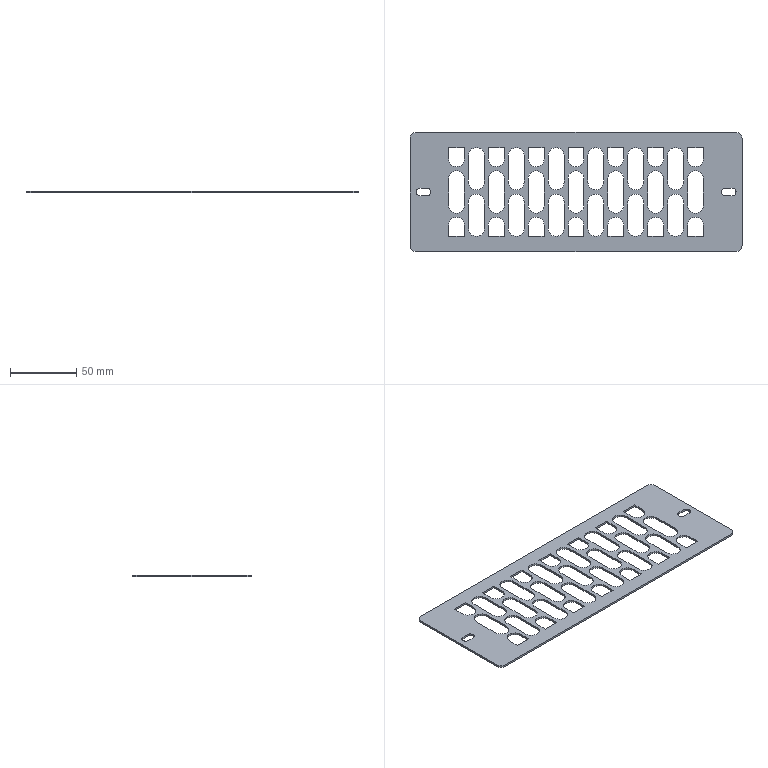Part | SolidWorks | features BaseBody 1 | 1 solid | 152 faces | box 250 x 90 x 1.5 mm | volume 20150 mm3 | plane 90 | cylinder 62 | commonest cylinder face diameters 12 x52 6 x6 10 x4